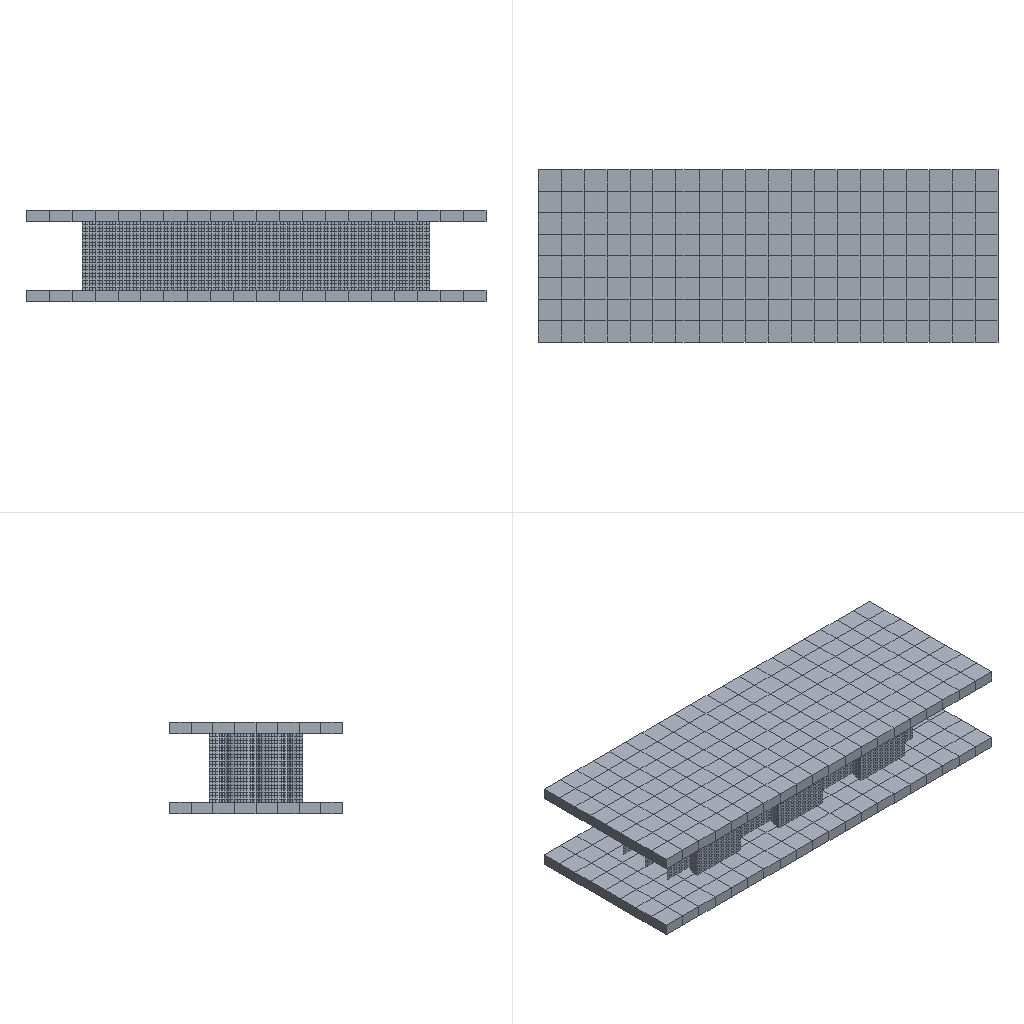Simulation study | abaqus
Set-up summary:
category,name,step,type,value,unit,region
solver,abaqus,,Abaqus/CAE 2024
units,mm-N-s-tonne (MPa),,inferred,E=70000 density=2.7e-09
analysis,Step-1,,dynamic explicit,nlgeom=True; time_period=0.01
mesh,nodes,,,15248
mesh,elements,,,15080
element_type,S4R,,,14760
element_type,C3D8R,,,320
material,Material-1,,E,70000
material,Material-1,,nu,0.33
material,Material-1,,density,2.7e-09
material,Material-1,,yield,276
material,Material-1,,behaviors,plastic
section,Material-1,,solid section,,,_PickedSet2
section,Material-1,,shell section,1,,_PickedSet4
bc,BC-1,initial,encastre,[dofs=ENCASTRE],,_PickedSet18
bc,BC-2,Step-1,fixed,"[dofs=rx,ry,rz,x,y n=5]",,_PickedSet19
bc,BC-2,Step-1,displacement,-3 [dofs=z],,_PickedSet19
contact,Int-1,initial,general contact,interaction=IntProp-1; friction=0.2; behavior=hard
constraint,rigid body,,,2
Abaqus input file, long lists of numbers shortened:
*Heading
** Job name: deck Model name: Model-1
** Generated by: Abaqus/CAE 2024
*Preprint, echo=NO, model=NO, history=NO, contact=NO
**
** PARTS
**
*Part, name=Part-2
*Node
      1,       -23.75,        -3.75,           1.
      2,       -23.75,       -1.875,           1.
** (376 more lines like these left out)
*Element, type=C3D8R
  1,  19,  20,  29,  28,   1,   2,  11,  10
  2,  20,  21,  30,  29,   2,   3,  12,  11
** (158 more lines like these left out)
*Nset, nset=_PickedSet2, internal, generate
   1,  378,    1
*Elset, elset=_PickedSet2, internal, generate
   1,  160,    1
** Section: Section-2
*Solid Section, elset=_PickedSet2, material=Material-1
,
*End Part
**
*Part, name=m-1
*Node
      1,   2.7,           0.,           0.
      2,   2.338,   1.35,           0.
** (14488 more lines like these left out)
*Element, type=S4R
  1,    1,   97, 2293,  142
  2,   97,   98, 2294, 2293
** (14758 more lines like these left out)
*Nset, nset=_PickedSet4, internal, generate
     1,  14490,      1
*Elset, elset=_PickedSet4, internal, generate
     1,  14760,      1
** Section: Section-1
*Shell Section, elset=_PickedSet4, material=Material-1
1., 5
*End Part
**
**
** ASSEMBLY
**
*Assembly, name=Assembly
**
*Instance, name=Part-2-1, part=Part-2
   18.864,        -6.45,           6.
*End Instance
**
*Instance, name=m-1-1, part=m-1
*End Instance
**
*Instance, name=Part-2-1-lin-2-1, part=Part-2
   18.864,        -6.45,          -1.
*End Instance
**
*Node
      1,   15.114,  -2.7,           7.
*Node
      2,   17.722,  -4.749,           0.
*Nset, nset=_PickedSet14, internal
 1,
*Nset, nset=_PickedSet15, internal, instance=Part-2-1, generate
   1,  378,    1
*Elset, elset=_PickedSet15, internal, instance=Part-2-1, generate
   1,  160,    1
*Nset, nset=_PickedSet16, internal
 2,
*Nset, nset=_PickedSet17, internal, instance=Part-2-1-lin-2-1, generate
   1,  378,    1
*Elset, elset=_PickedSet17, internal, instance=Part-2-1-lin-2-1, generate
   1,  160,    1
*Nset, nset=_PickedSet18, internal
 2,
*Nset, nset=_PickedSet19, internal
 1,
** Constraint: Constraint-1
*Rigid Body, ref node=_PickedSet14, elset=_PickedSet15
** Constraint: Constraint-2
*Rigid Body, ref node=_PickedSet16, elset=_PickedSet17
*End Assembly
*Amplitude, name=Amp-1
             0.,              0.,            0.01,              1.
**
** MATERIALS
**
*Material, name=Material-1
*Density
 2.7e-09,
*Elastic
70000., 0.33
*Plastic
  276.,     0.
 296.5, 0.0052
  310., 0.0138
  324., 0.0308
 338.5, 0.0613
  345.,    0.1
**
** INTERACTION PROPERTIES
**
*Surface Interaction, name=IntProp-1
*Friction
 0.2,
*Surface Behavior, pressure-overclosure=HARD
**
** BOUNDARY CONDITIONS
**
** Name: BC-1 Type: Symmetry/Antisymmetry/Encastre
*Boundary
_PickedSet18, ENCASTRE
**
** INTERACTIONS
**
** Interaction: Int-1
*Contact, op=NEW
*Contact Inclusions, ALL EXTERIOR
*Contact Property Assignment
 ,  , IntProp-1
** ----------------------------------------------------------------
**
** STEP: Step-1
**
*Step, name=Step-1, nlgeom=YES
*Dynamic, Explicit
, 0.01
*Bulk Viscosity
0.06, 1.2
** Mass Scaling: Semi-Automatic
**               Whole Model
*Fixed Mass Scaling, factor=1000.
**
** BOUNDARY CONDITIONS
**
** Name: BC-2 Type: Displacement/Rotation
*Boundary, amplitude=Amp-1
_PickedSet19, 1, 1
_PickedSet19, 2, 2
_PickedSet19, 3, 3, -3.
_PickedSet19, 4, 4
_PickedSet19, 5, 5
_PickedSet19, 6, 6
**
** OUTPUT REQUESTS
**
*Restart, write, number interval=1, time marks=NO
**
** FIELD OUTPUT: F-Output-1
**
*Output, field, variable=PRESELECT, number interval=50
**
** HISTORY OUTPUT: H-Output-1
**
*Output, history, variable=PRESELECT
*End Step
Results summary:
result,odb.job_status,,,JOB_STATUS_UNKNOWN,"consistent, unstated (Abaqus has no unit system)"
result,steps[0].procedure,Step-1,,"*DYNAMIC, EXPLICIT","consistent, unstated (Abaqus has no unit system)"
result,steps[0].time_period,Step-1,,0.01,"consistent, unstated (Abaqus has no unit system)"
result,steps[0].n_frames,Step-1,,50,"consistent, unstated (Abaqus has no unit system)"
result,steps[0].last_frame.id,Step-1,,22658,"consistent, unstated (Abaqus has no unit system)"
result,steps[0].last_frame.value,Step-1,,0.0098,"consistent, unstated (Abaqus has no unit system)"
result,steps[0].last_frame.description,Step-1,,Increment     22658: Step Time =   9.8001E-03,"consistent, unstated (Abaqus has no unit system)"
result,steps[0].completed,Step-1,,False,"consistent, unstated (Abaqus has no unit system)"
result,steps[0].max_U_magnitude,Step-1,,3.144,"consistent, unstated (Abaqus has no unit system)"
result,steps[0].max_S_mises,Step-1,,345,"consistent, unstated (Abaqus has no unit system)"
result,steps[0].RF_sum[1],Step-1,,-42.264,"consistent, unstated (Abaqus has no unit system)"
result,steps[0].RF_sum[2],Step-1,,141.154,"consistent, unstated (Abaqus has no unit system)"
result,steps[0].RF_sum[3],Step-1,,10.438,"consistent, unstated (Abaqus has no unit system)"
result,steps[0].diagnostic.n_increments,Step-1,,50,"consistent, unstated (Abaqus has no unit system)"